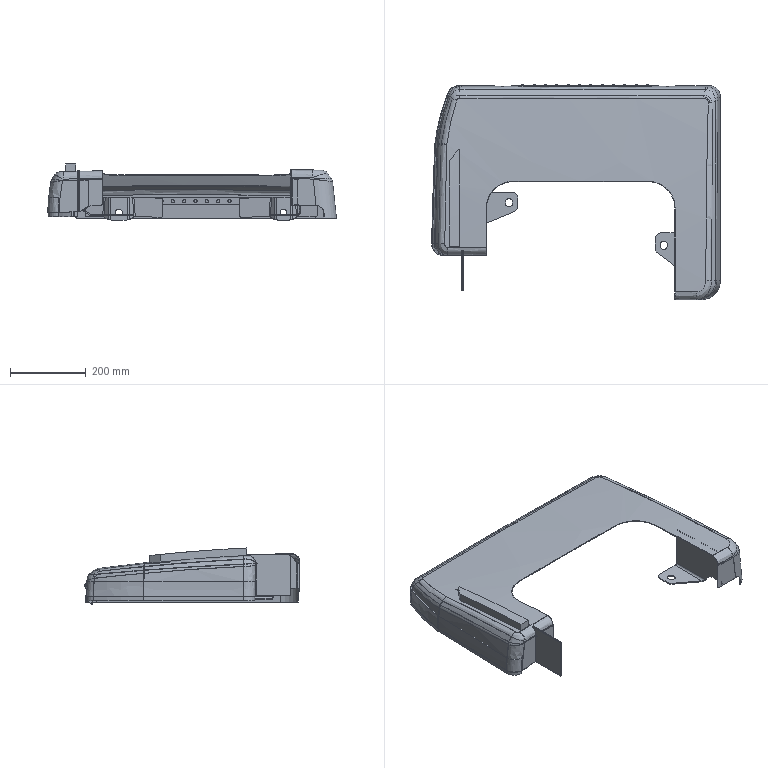Part | SolidWorks | features BaseBody 10 | 10 solids | 675 faces | box 763.446 x 569.652 x 148.304 mm | volume 1530854 mm3 | spline 211 | plane 210 | cylinder 146 | cone 60 | torus 48 | commonest cylinder face diameters 10 x29 3.2 x25 3 x24 60 x21 16.4 x13 18 x8